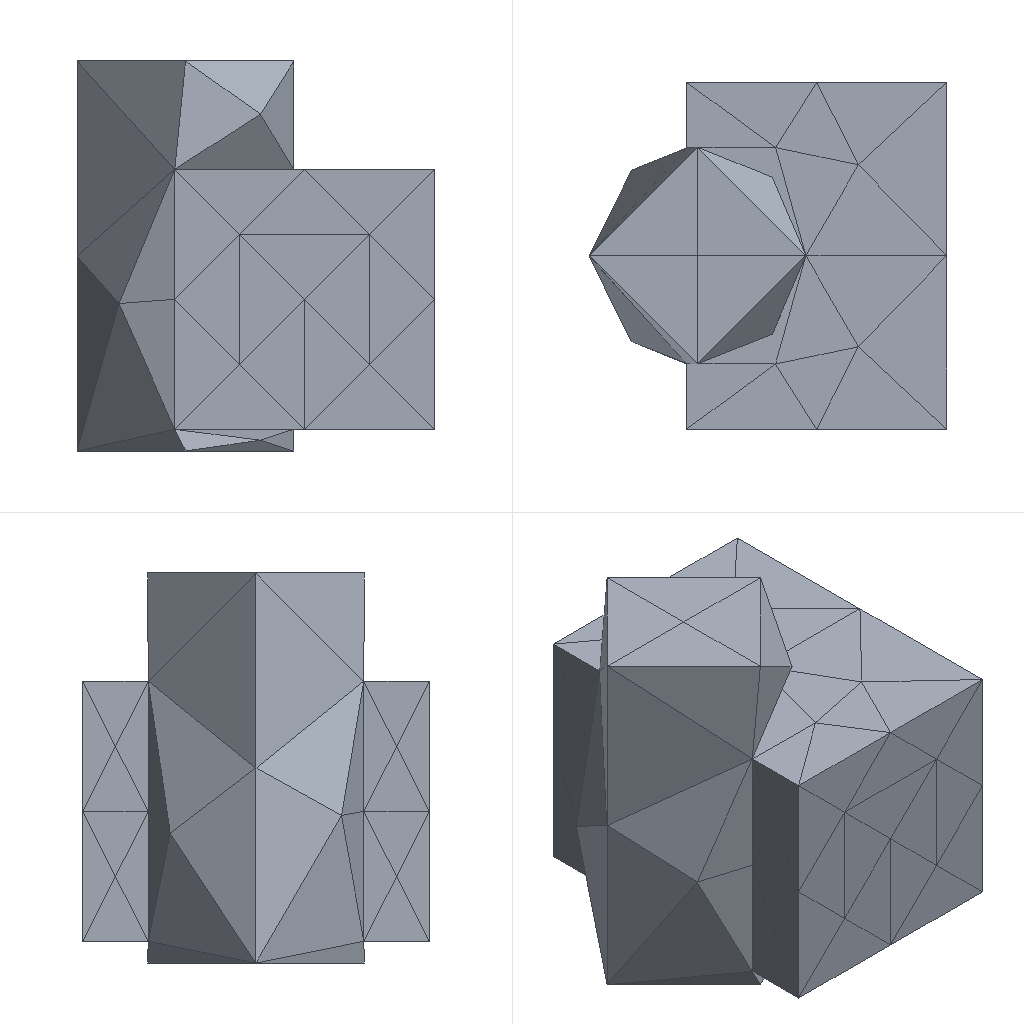Simulation study | ansys mapdl
Set-up summary:
category,name,step,type,value,unit,region
solver,ansys_mapdl
units,mm-N-s-tonne (MPa),,inferred,E=210000 density=
analysis,model,,static
mesh,nodes,,,438
mesh,elements,,,214
element_type,SOLID187,,,214
material,mat 1,,E,210000
material,mat 1,,nu,0.3
load,,model,body load temp,,,all
load,,model,force,"1000 [dir=(0, 0, -1) n=33]",,node list
bc,,model,fixed,"[dofs=UX,UY,UZ n=564]",,node list
Ansys APDL input file, long lists of numbers shortened:
/COM,ANSYS RELEASE 2026 R1           BUILD 26.1      UP20260202       09:09:57
/PREP7
/NOPR
/TITLE,2
ANTYPE, 0
*IF,_CDRDOFF,EQ,1,THEN     !if solid model was read in
_CDRDOFF=             !reset flag, numoffs already performed
*ELSE              !offset database for the following FE model
NUMOFF,NODE,      438
NUMOFF,ELEM,      214
NUMOFF,MAT ,        1
NUMOFF,TYPE,        1
*ENDIF
*SET,_RETURN ,  0.
*SET,_STATUS ,  0.
*SET,_UIQR   ,  33.
*SET,__FLOATPARAMETER__,  438.
DOF,DELETE
ETBLOCK,        1,        1
(2i9,19a9)
        1      187        0        0        0        0        0        0        0        0        0        0        0        0        0        0        0        0        0        0        0
       -1
NBLOCK,6,SOLID,       438,       438
(3i9,6e21.13e3)
        1        0        0 3.8500000000000E+001 6.1232339957368E-016-1.0000000000000E+000
! (437 more lines like these left out)
N,UNBL,LOC,       -1,
EBLOCK,19,SOLID,       214,       214
(19i10)
         1         1         1         1         0         0         0         0        10         0         1       205       114       112       143       198       113       200       281
! (427 more lines like these left out)
        -1
MPTEMP,UNBL, 1, 1,  0.    ,
MPDATA,UNBL, 1,EX  ,       1, 1,  210000.000    ,
MPTEMP,UNBL, 1, 1,  0.    ,
MPDATA,UNBL, 1,NUXY,       1, 1, 0.3    ,
MPTEMP,UNBL, 1, 1,  0.    ,
MPDATA,UNBL, 1,PRXY,       1, 1, 0.3    ,
EXTOPT,ATTR,      0,      0,      0
EXTOPT,ESIZE,  0,  0.
EXTOPT,ACLEAR,      0
TREF,  0.
IRLF,  0
BFUNIF,TEMP,_TINY
ACEL,  0.    ,  0.    ,  0.
OMEGA,  0.    ,  0.    ,  0.
DOMEGA,  0.    ,  0.    ,  0.
CGLOC,  0.    ,  0.    ,  0.
CGOMEGA,  0.    ,  0.    ,  0.
DCGOMG,  0.    ,  0.    ,  0.
KUSE,     0
TIME,  0.
ALPHAD,  0.
BETAD,  0.
DMPRAT,  0.
DMPSTR,  0.
CRPLIM, 0.1    ,   0
CRPLIM,  0.    ,   1
NCNV,     0, 1.000000000E+12,     0,  0.    ,  0.
NEQIT,     0
ERESX,DEFA
DBLOCK,       564
(i9,a6,2(pg16.9))
        1  UX    0.00000000      0.00000000
! (563 more lines like these left out)
       -1
FBLOCK,        33
(i9,a6,2(pg16.9))
       16  FZ   -30.3030303      0.00000000
! (32 more lines like these left out)
       -1
/GO
FINISH
Results summary:
result,analysis_type_db,,,static,unstated
result,n_sets,,,1,unstated
result,load_steps[0].set,load_step=1,,1,unstated
result,load_steps[0].substep,load_step=1,,1,unstated
result,load_steps[0].time,load_step=1,,1,unstated
result,load_steps[0].freq,load_step=1,,1,unstated
result,load_steps[0].max_usum,load_step=1,,0.001026,unstated
result,load_steps[0].max_seqv,load_step=1,,21.856,unstated
result,load_steps[0].reaction_sum.FX,load_step=1,,1.65556e-11,unstated
result,load_steps[0].reaction_sum.FY,load_step=1,,5.09526e-12,unstated
result,load_steps[0].reaction_sum.FZ,load_step=1,,1000,unstated
result,load_steps[0].reaction_sum.MX,load_step=1,,0,unstated
result,load_steps[0].reaction_sum.MY,load_step=1,,0,unstated
result,load_steps[0].reaction_sum.MZ,load_step=1,,0,unstated
result,convergence,,,results present for all listed sets,unstated